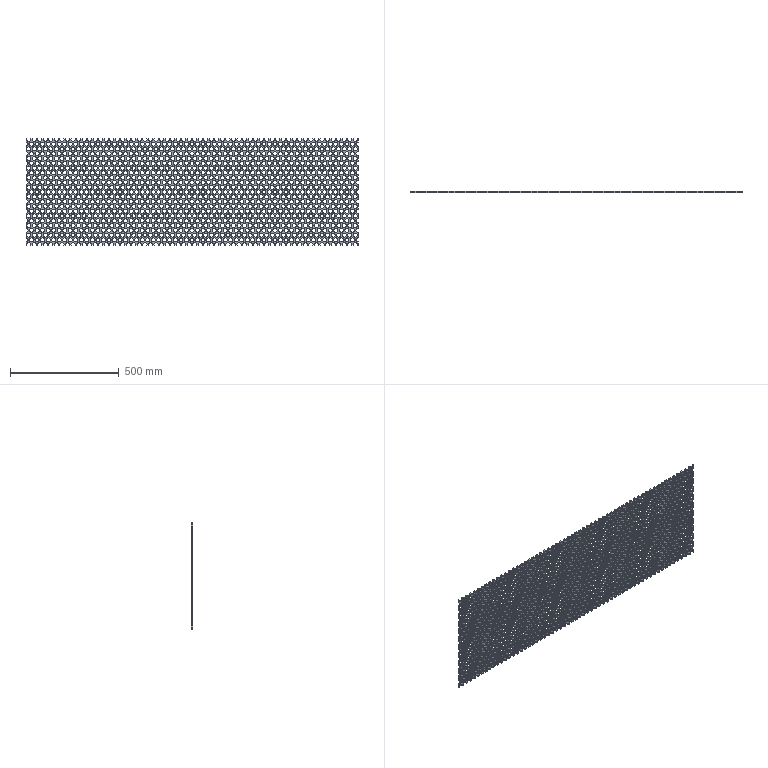Part | 1 solid | 2788 faces | box 1524 x 6 x 490 mm | volume 2182298 mm3 | cylinder 2640 | plane 148 | commonest cylinder face diameters 19.05 x2640